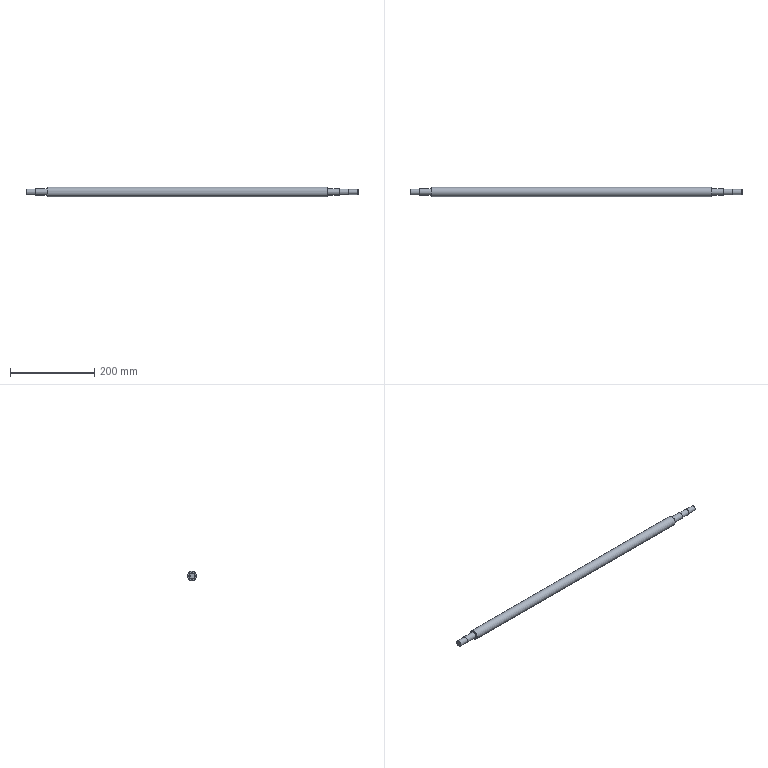Part | NX | 1 solid | 28 faces | box 787 x 22 x 22 mm | volume 271373 mm3 | plane 13 | cylinder 10 | cone 5 | commonest cylinder face diameters 5 x4 14 x2 15 x2 12 x1 22 x1
STEP:
#1=CARTESIAN_POINT('',(382.5,0.,-6.5));
#2=VERTEX_POINT('',#1);
#3=CARTESIAN_POINT('',(382.5,0.,0.));
#4=DIRECTION('',(1.,0.,0.));
#5=DIRECTION('',(0.,0.,-1.));
#6=AXIS2_PLACEMENT_3D('',#3,#4,#5);
#7=CIRCLE('',#6,6.5);
#8=EDGE_CURVE('',#2,#2,#7,.T.);
#9=ORIENTED_EDGE('',*,*,#8,.T.);
#10=EDGE_LOOP('',(#9));
#11=FACE_BOUND('',#10,.T.);
#12=CARTESIAN_POINT('',(382.5,0.,-6.));
#13=VERTEX_POINT('',#12);
#14=CARTESIAN_POINT('',(382.5,0.,0.));
#15=DIRECTION('',(1.,0.,0.));
#16=DIRECTION('',(0.,0.,-1.));
#17=AXIS2_PLACEMENT_3D('',#14,#15,#16);
#18=CIRCLE('',#17,6.);
#19=EDGE_CURVE('',#13,#13,#18,.T.);
#20=ORIENTED_EDGE('',*,*,#19,.F.);
#21=EDGE_LOOP('',(#20));
#22=FACE_BOUND('',#21,.T.);
#23=CARTESIAN_POINT('',(382.5,0.,0.));
#24=DIRECTION('',(1.,0.,0.));
#25=DIRECTION('',(0.,0.,-1.));
#26=AXIS2_PLACEMENT_3D('',#23,#24,#25);
#27=PLANE('',#26);
#28=ADVANCED_FACE('',(#11,#22),#27,.T.);
#29=CARTESIAN_POINT('',(382.,0.,-7.));
#30=VERTEX_POINT('',#29);
#31=CARTESIAN_POINT('',(382.,0.,0.));
#32=DIRECTION('',(1.,0.,0.));
#33=DIRECTION('',(0.,0.,-1.));
#34=AXIS2_PLACEMENT_3D('',#31,#32,#33);
#35=CIRCLE('',#34,7.);
#36=EDGE_CURVE('',#30,#30,#35,.F.);
#37=ORIENTED_EDGE('',*,*,#36,.T.);
#38=EDGE_LOOP('',(#37));
#39=FACE_BOUND('',#38,.T.);
#40=CARTESIAN_POINT('',(360.5,0.,-7.));
#41=VERTEX_POINT('',#40);
#42=CARTESIAN_POINT('',(360.5,0.,0.));
#43=DIRECTION('',(1.,0.,0.));
#44=DIRECTION('',(0.,0.,-1.));
#45=AXIS2_PLACEMENT_3D('',#42,#43,#44);
#46=CIRCLE('',#45,7.);
#47=EDGE_CURVE('',#41,#41,#46,.T.);
#48=ORIENTED_EDGE('',*,*,#47,.T.);
#49=EDGE_LOOP('',(#48));
#50=FACE_BOUND('',#49,.T.);
#51=CARTESIAN_POINT('',(363.5,6.538,-2.5));
#52=VERTEX_POINT('',#51);
#53=CARTESIAN_POINT('',(363.5,6.538,2.5));
#54=VERTEX_POINT('',#53);
#55=CARTESIAN_POINT('',(363.5,6.538,-2.5));
#56=CARTESIAN_POINT('',(362.834,6.538,-2.5));
#57=CARTESIAN_POINT('',(361.548,6.777,-1.958));
#58=CARTESIAN_POINT('',(360.726,7.111,-0.004587));
#59=CARTESIAN_POINT('',(361.547,6.777,1.96));
#60=CARTESIAN_POINT('',(362.833,6.538,2.5));
#61=CARTESIAN_POINT('',(363.5,6.538,2.5));
#62=B_SPLINE_CURVE_WITH_KNOTS('',3,(#55,#56,#57,#58,#59,#60,#61),.UNSPECIFIED.,.F.,.F.,(4,1,1,1,4),(0.,0.00197,0.003939,0.005909,0.007878),.UNSPECIFIED.);
#63=EDGE_CURVE('',#52,#54,#62,.T.);
#64=ORIENTED_EDGE('',*,*,#63,.F.);
#65=CARTESIAN_POINT('',(378.5,6.538,-2.5));
#66=VERTEX_POINT('',#65);
#67=CARTESIAN_POINT('',(382.5,6.538,-2.5));
#68=DIRECTION('',(-1.,0.,0.));
#69=VECTOR('',#68,1000.);
#70=LINE('',#67,#69);
#71=EDGE_CURVE('',#66,#52,#70,.T.);
#72=ORIENTED_EDGE('',*,*,#71,.F.);
#73=CARTESIAN_POINT('',(378.5,6.538,2.5));
#74=VERTEX_POINT('',#73);
#75=CARTESIAN_POINT('',(378.5,6.538,2.5));
#76=CARTESIAN_POINT('',(379.166,6.538,2.5));
#77=CARTESIAN_POINT('',(380.452,6.777,1.958));
#78=CARTESIAN_POINT('',(381.274,7.111,0.004587));
#79=CARTESIAN_POINT('',(380.453,6.777,-1.96));
#80=CARTESIAN_POINT('',(379.167,6.538,-2.5));
#81=CARTESIAN_POINT('',(378.5,6.538,-2.5));
#82=B_SPLINE_CURVE_WITH_KNOTS('',3,(#75,#76,#77,#78,#79,#80,#81),.UNSPECIFIED.,.F.,.F.,(4,1,1,1,4),(0.,0.00197,0.003939,0.005909,0.007878),.UNSPECIFIED.);
#83=EDGE_CURVE('',#74,#66,#82,.T.);
#84=ORIENTED_EDGE('',*,*,#83,.F.);
#85=CARTESIAN_POINT('',(382.5,6.538,2.5));
#86=DIRECTION('',(-1.,0.,0.));
#87=VECTOR('',#86,1000.);
#88=LINE('',#85,#87);
#89=EDGE_CURVE('',#54,#74,#88,.F.);
#90=ORIENTED_EDGE('',*,*,#89,.F.);
#91=EDGE_LOOP('',(#64,#72,#84,#90));
#92=FACE_BOUND('',#91,.T.);
#93=CARTESIAN_POINT('',(382.5,0.,0.));
#94=DIRECTION('',(-1.,0.,0.));
#95=DIRECTION('',(0.,0.,1.));
#96=AXIS2_PLACEMENT_3D('',#93,#94,#95);
#97=CYLINDRICAL_SURFACE('',#96,7.);
#98=ADVANCED_FACE('',(#39,#50,#92),#97,.T.);
#99=CARTESIAN_POINT('',(360.5,0.,-7.5));
#100=VERTEX_POINT('',#99);
#101=CARTESIAN_POINT('',(360.5,0.,0.));
#102=DIRECTION('',(1.,0.,0.));
#103=DIRECTION('',(0.,0.,-1.));
#104=AXIS2_PLACEMENT_3D('',#101,#102,#103);
#105=CIRCLE('',#104,7.5);
#106=EDGE_CURVE('',#100,#100,#105,.T.);
#107=ORIENTED_EDGE('',*,*,#106,.T.);
#108=EDGE_LOOP('',(#107));
#109=FACE_BOUND('',#108,.T.);
#110=ORIENTED_EDGE('',*,*,#47,.F.);
#111=EDGE_LOOP('',(#110));
#112=FACE_BOUND('',#111,.T.);
#113=CARTESIAN_POINT('',(360.5,0.,0.));
#114=DIRECTION('',(1.,0.,0.));
#115=DIRECTION('',(0.,0.,-1.));
#116=AXIS2_PLACEMENT_3D('',#113,#114,#115);
#117=PLANE('',#116);
#118=ADVANCED_FACE('',(#109,#112),#117,.T.);
#119=CARTESIAN_POINT('',(332.5,0.,-10.5));
#120=VERTEX_POINT('',#119);
#121=CARTESIAN_POINT('',(332.5,0.,0.));
#122=DIRECTION('',(1.,0.,0.));
#123=DIRECTION('',(0.,0.,-1.));
#124=AXIS2_PLACEMENT_3D('',#121,#122,#123);
#125=CIRCLE('',#124,10.5);
#126=EDGE_CURVE('',#120,#120,#125,.T.);
#127=ORIENTED_EDGE('',*,*,#126,.T.);
#128=EDGE_LOOP('',(#127));
#129=FACE_BOUND('',#128,.T.);
#130=CARTESIAN_POINT('',(332.5,0.,-7.5));
#131=VERTEX_POINT('',#130);
#132=CARTESIAN_POINT('',(332.5,0.,0.));
#133=DIRECTION('',(1.,0.,0.));
#134=DIRECTION('',(0.,0.,-1.));
#135=AXIS2_PLACEMENT_3D('',#132,#133,#134);
#136=CIRCLE('',#135,7.5);
#137=EDGE_CURVE('',#131,#131,#136,.T.);
#138=ORIENTED_EDGE('',*,*,#137,.F.);
#139=EDGE_LOOP('',(#138));
#140=FACE_BOUND('',#139,.T.);
#141=CARTESIAN_POINT('',(332.5,0.,0.));
#142=DIRECTION('',(1.,0.,0.));
#143=DIRECTION('',(0.,0.,-1.));
#144=AXIS2_PLACEMENT_3D('',#141,#142,#143);
#145=PLANE('',#144);
#146=ADVANCED_FACE('',(#129,#140),#145,.T.);
#147=CARTESIAN_POINT('',(-332.,0.,-11.));
#148=VERTEX_POINT('',#147);
#149=CARTESIAN_POINT('',(-332.,0.,0.));
#150=DIRECTION('',(1.,0.,0.));
#151=DIRECTION('',(0.,0.,-1.));
#152=AXIS2_PLACEMENT_3D('',#149,#150,#151);
#153=CIRCLE('',#152,11.);
#154=EDGE_CURVE('',#148,#148,#153,.T.);
#155=ORIENTED_EDGE('',*,*,#154,.T.);
#156=EDGE_LOOP('',(#155));
#157=FACE_BOUND('',#156,.T.);
#158=CARTESIAN_POINT('',(332.,0.,-11.));
#159=VERTEX_POINT('',#158);
#160=CARTESIAN_POINT('',(332.,0.,0.));
#161=DIRECTION('',(1.,0.,0.));
#162=DIRECTION('',(0.,0.,-1.));
#163=AXIS2_PLACEMENT_3D('',#160,#161,#162);
#164=CIRCLE('',#163,11.);
#165=EDGE_CURVE('',#159,#159,#164,.F.);
#166=ORIENTED_EDGE('',*,*,#165,.T.);
#167=EDGE_LOOP('',(#166));
#168=FACE_BOUND('',#167,.T.);
#169=CARTESIAN_POINT('',(332.5,0.,0.));
#170=DIRECTION('',(-1.,0.,0.));
#171=DIRECTION('',(0.,0.,1.));
#172=AXIS2_PLACEMENT_3D('',#169,#170,#171);
#173=CYLINDRICAL_SURFACE('',#172,11.);
#174=ADVANCED_FACE('',(#157,#168),#173,.T.);
#175=CARTESIAN_POINT('',(-332.5,0.,-10.5));
#176=VERTEX_POINT('',#175);
#177=CARTESIAN_POINT('',(-332.5,0.,0.));
#178=DIRECTION('',(1.,0.,0.));
#179=DIRECTION('',(0.,0.,-1.));
#180=AXIS2_PLACEMENT_3D('',#177,#178,#179);
#181=CIRCLE('',#180,10.5);
#182=EDGE_CURVE('',#176,#176,#181,.F.);
#183=ORIENTED_EDGE('',*,*,#182,.T.);
#184=EDGE_LOOP('',(#183));
#185=FACE_BOUND('',#184,.T.);
#186=CARTESIAN_POINT('',(-332.5,0.,-7.5));
#187=VERTEX_POINT('',#186);
#188=CARTESIAN_POINT('',(-332.5,0.,0.));
#189=DIRECTION('',(1.,0.,0.));
#190=DIRECTION('',(0.,0.,-1.));
#191=AXIS2_PLACEMENT_3D('',#188,#189,#190);
#192=CIRCLE('',#191,7.5);
#193=EDGE_CURVE('',#187,#187,#192,.T.);
#194=ORIENTED_EDGE('',*,*,#193,.T.);
#195=EDGE_LOOP('',(#194));
#196=FACE_BOUND('',#195,.T.);
#197=CARTESIAN_POINT('',(-332.5,0.,0.));
#198=DIRECTION('',(1.,0.,0.));
#199=DIRECTION('',(0.,0.,-1.));
#200=AXIS2_PLACEMENT_3D('',#197,#198,#199);
#201=PLANE('',#200);
#202=ADVANCED_FACE('',(#185,#196),#201,.F.);
#203=ORIENTED_EDGE('',*,*,#106,.F.);
#204=EDGE_LOOP('',(#203));
#205=FACE_BOUND('',#204,.T.);
#206=ORIENTED_EDGE('',*,*,#137,.T.);
#207=EDGE_LOOP('',(#206));
#208=FACE_BOUND('',#207,.T.);
#209=CARTESIAN_POINT('',(360.5,0.,0.));
#210=DIRECTION('',(-1.,0.,0.));
#211=DIRECTION('',(0.,0.,1.));
#212=AXIS2_PLACEMENT_3D('',#209,#210,#211);
#213=CYLINDRICAL_SURFACE('',#212,7.5);
#214=ADVANCED_FACE('',(#205,#208),#213,.T.);
#215=CARTESIAN_POINT('',(378.5,4.,2.5));
#216=VERTEX_POINT('',#215);
#217=CARTESIAN_POINT('',(378.5,4.,2.5));
#218=DIRECTION('',(0.,1.,0.));
#219=VECTOR('',#218,1000.);
#220=LINE('',#217,#219);
#221=EDGE_CURVE('',#216,#74,#220,.T.);
#222=ORIENTED_EDGE('',*,*,#221,.T.);
#223=ORIENTED_EDGE('',*,*,#83,.T.);
#224=CARTESIAN_POINT('',(378.5,4.,-2.5));
#225=VERTEX_POINT('',#224);
#226=CARTESIAN_POINT('',(378.5,4.,-2.5));
#227=DIRECTION('',(0.,1.,0.));
#228=VECTOR('',#227,1000.);
#229=LINE('',#226,#228);
#230=EDGE_CURVE('',#225,#66,#229,.T.);
#231=ORIENTED_EDGE('',*,*,#230,.F.);
#232=CARTESIAN_POINT('',(378.5,4.,0.));
#233=DIRECTION('',(0.,-1.,0.));
#234=DIRECTION('',(0.,0.,1.));
#235=AXIS2_PLACEMENT_3D('',#232,#233,#234);
#236=CIRCLE('',#235,2.5);
#237=EDGE_CURVE('',#225,#216,#236,.T.);
#238=ORIENTED_EDGE('',*,*,#237,.T.);
#239=EDGE_LOOP('',(#222,#223,#231,#238));
#240=FACE_BOUND('',#239,.T.);
#241=CARTESIAN_POINT('',(378.5,4.,0.));
#242=DIRECTION('',(0.,1.,0.));
#243=DIRECTION('',(0.,0.,1.));
#244=AXIS2_PLACEMENT_3D('',#241,#242,#243);
#245=CYLINDRICAL_SURFACE('',#244,2.5);
#246=ADVANCED_FACE('',(#240),#245,.F.);
#247=ORIENTED_EDGE('',*,*,#89,.T.);
#248=ORIENTED_EDGE('',*,*,#221,.F.);
#249=CARTESIAN_POINT('',(363.5,4.,2.5));
#250=VERTEX_POINT('',#249);
#251=CARTESIAN_POINT('',(378.5,4.,2.5));
#252=DIRECTION('',(-1.,0.,0.));
#253=VECTOR('',#252,1000.);
#254=LINE('',#251,#253);
#255=EDGE_CURVE('',#216,#250,#254,.T.);
#256=ORIENTED_EDGE('',*,*,#255,.T.);
#257=CARTESIAN_POINT('',(363.5,4.,2.5));
#258=DIRECTION('',(0.,1.,0.));
#259=VECTOR('',#258,1000.);
#260=LINE('',#257,#259);
#261=EDGE_CURVE('',#250,#54,#260,.T.);
#262=ORIENTED_EDGE('',*,*,#261,.T.);
#263=EDGE_LOOP('',(#247,#248,#256,#262));
#264=FACE_BOUND('',#263,.T.);
#265=CARTESIAN_POINT('',(378.5,4.,2.5));
#266=DIRECTION('',(0.,0.,-1.));
#267=DIRECTION('',(0.,1.,0.));
#268=AXIS2_PLACEMENT_3D('',#265,#266,#267);
#269=PLANE('',#268);
#270=ADVANCED_FACE('',(#264),#269,.T.);
#271=CARTESIAN_POINT('',(363.5,4.,-2.5));
#272=VERTEX_POINT('',#271);
#273=CARTESIAN_POINT('',(363.5,4.,-2.5));
#274=DIRECTION('',(0.,1.,0.));
#275=VECTOR('',#274,1000.);
#276=LINE('',#273,#275);
#277=EDGE_CURVE('',#272,#52,#276,.T.);
#278=ORIENTED_EDGE('',*,*,#277,.T.);
#279=ORIENTED_EDGE('',*,*,#63,.T.);
#280=ORIENTED_EDGE('',*,*,#261,.F.);
#281=CARTESIAN_POINT('',(363.5,4.,0.));
#282=DIRECTION('',(0.,-1.,0.));
#283=DIRECTION('',(0.,0.,-1.));
#284=AXIS2_PLACEMENT_3D('',#281,#282,#283);
#285=CIRCLE('',#284,2.5);
#286=EDGE_CURVE('',#250,#272,#285,.T.);
#287=ORIENTED_EDGE('',*,*,#286,.T.);
#288=EDGE_LOOP('',(#278,#279,#280,#287));
#289=FACE_BOUND('',#288,.T.);
#290=CARTESIAN_POINT('',(363.5,4.,0.));
#291=DIRECTION('',(0.,1.,0.));
#292=DIRECTION('',(0.,0.,1.));
#293=AXIS2_PLACEMENT_3D('',#290,#291,#292);
#294=CYLINDRICAL_SURFACE('',#293,2.5);
#295=ADVANCED_FACE('',(#289),#294,.F.);
#296=ORIENTED_EDGE('',*,*,#71,.T.);
#297=ORIENTED_EDGE('',*,*,#277,.F.);
#298=CARTESIAN_POINT('',(378.5,4.,-2.5));
#299=DIRECTION('',(1.,0.,0.));
#300=VECTOR('',#299,1000.);
#301=LINE('',#298,#300);
#302=EDGE_CURVE('',#272,#225,#301,.T.);
#303=ORIENTED_EDGE('',*,*,#302,.T.);
#304=ORIENTED_EDGE('',*,*,#230,.T.);
#305=EDGE_LOOP('',(#296,#297,#303,#304));
#306=FACE_BOUND('',#305,.T.);
#307=CARTESIAN_POINT('',(378.5,4.,-2.5));
#308=DIRECTION('',(0.,0.,1.));
#309=DIRECTION('',(0.,-1.,0.));
#310=AXIS2_PLACEMENT_3D('',#307,#308,#309);
#311=PLANE('',#310);
#312=ADVANCED_FACE('',(#306),#311,.T.);
#313=ORIENTED_EDGE('',*,*,#237,.F.);
#314=ORIENTED_EDGE('',*,*,#302,.F.);
#315=ORIENTED_EDGE('',*,*,#286,.F.);
#316=ORIENTED_EDGE('',*,*,#255,.F.);
#317=EDGE_LOOP('',(#313,#314,#315,#316));
#318=FACE_BOUND('',#317,.T.);
#319=CARTESIAN_POINT('',(378.5,4.,0.));
#320=DIRECTION('',(0.,1.,0.));
#321=DIRECTION('',(0.,0.,1.));
#322=AXIS2_PLACEMENT_3D('',#319,#320,#321);
#323=PLANE('',#322);
#324=ADVANCED_FACE('',(#318),#323,.T.);
#325=CARTESIAN_POINT('',(-360.5,0.,-7.5));
#326=VERTEX_POINT('',#325);
#327=CARTESIAN_POINT('',(-360.5,0.,0.));
#328=DIRECTION('',(1.,0.,0.));
#329=DIRECTION('',(0.,0.,-1.));
#330=AXIS2_PLACEMENT_3D('',#327,#328,#329);
#331=CIRCLE('',#330,7.5);
#332=EDGE_CURVE('',#326,#326,#331,.T.);
#333=ORIENTED_EDGE('',*,*,#332,.T.);
#334=EDGE_LOOP('',(#333));
#335=FACE_BOUND('',#334,.T.);
#336=ORIENTED_EDGE('',*,*,#193,.F.);
#337=EDGE_LOOP('',(#336));
#338=FACE_BOUND('',#337,.T.);
#339=CARTESIAN_POINT('',(-360.5,0.,0.));
#340=DIRECTION('',(1.,0.,0.));
#341=DIRECTION('',(0.,0.,-1.));
#342=AXIS2_PLACEMENT_3D('',#339,#340,#341);
#343=CYLINDRICAL_SURFACE('',#342,7.5);
#344=ADVANCED_FACE('',(#335,#338),#343,.T.);
#345=CARTESIAN_POINT('',(-360.5,0.,7.));
#346=VERTEX_POINT('',#345);
#347=CARTESIAN_POINT('',(-360.5,0.,0.));
#348=DIRECTION('',(-1.,0.,0.));
#349=DIRECTION('',(0.,0.,1.));
#350=AXIS2_PLACEMENT_3D('',#347,#348,#349);
#351=CIRCLE('',#350,7.);
#352=EDGE_CURVE('',#346,#346,#351,.T.);
#353=ORIENTED_EDGE('',*,*,#352,.F.);
#354=EDGE_LOOP('',(#353));
#355=FACE_BOUND('',#354,.T.);
#356=ORIENTED_EDGE('',*,*,#332,.F.);
#357=EDGE_LOOP('',(#356));
#358=FACE_BOUND('',#357,.T.);
#359=CARTESIAN_POINT('',(-360.5,0.,0.));
#360=DIRECTION('',(-1.,0.,0.));
#361=DIRECTION('',(0.,0.,-1.));
#362=AXIS2_PLACEMENT_3D('',#359,#360,#361);
#363=PLANE('',#362);
#364=ADVANCED_FACE('',(#355,#358),#363,.T.);
#365=CARTESIAN_POINT('',(-382.,0.,7.));
#366=VERTEX_POINT('',#365);
#367=CARTESIAN_POINT('',(-382.,0.,0.));
#368=DIRECTION('',(-1.,0.,0.));
#369=DIRECTION('',(0.,0.,1.));
#370=AXIS2_PLACEMENT_3D('',#367,#368,#369);
#371=CIRCLE('',#370,7.);
#372=EDGE_CURVE('',#366,#366,#371,.F.);
#373=ORIENTED_EDGE('',*,*,#372,.T.);
#374=EDGE_LOOP('',(#373));
#375=FACE_BOUND('',#374,.T.);
#376=CARTESIAN_POINT('',(-363.5,6.538,2.5));
#377=VERTEX_POINT('',#376);
#378=CARTESIAN_POINT('',(-363.5,6.538,-2.5));
#379=VERTEX_POINT('',#378);
#380=CARTESIAN_POINT('',(-363.5,6.538,2.5));
#381=CARTESIAN_POINT('',(-362.834,6.538,2.5));
#382=CARTESIAN_POINT('',(-361.548,6.777,1.958));
#383=CARTESIAN_POINT('',(-360.726,7.111,0.004587));
#384=CARTESIAN_POINT('',(-361.547,6.777,-1.96));
#385=CARTESIAN_POINT('',(-362.833,6.538,-2.5));
#386=CARTESIAN_POINT('',(-363.5,6.538,-2.5));
#387=B_SPLINE_CURVE_WITH_KNOTS('',3,(#380,#381,#382,#383,#384,#385,#386),.UNSPECIFIED.,.F.,.F.,(4,1,1,1,4),(0.,0.00197,0.003939,0.005909,0.007878),.UNSPECIFIED.);
#388=EDGE_CURVE('',#377,#379,#387,.T.);
#389=ORIENTED_EDGE('',*,*,#388,.F.);
#390=CARTESIAN_POINT('',(-378.5,6.538,2.5));
#391=VERTEX_POINT('',#390);
#392=CARTESIAN_POINT('',(-382.5,6.538,2.5));
#393=DIRECTION('',(1.,0.,0.));
#394=VECTOR('',#393,1000.);
#395=LINE('',#392,#394);
#396=EDGE_CURVE('',#391,#377,#395,.T.);
#397=ORIENTED_EDGE('',*,*,#396,.F.);
#398=CARTESIAN_POINT('',(-378.5,6.538,-2.5));
#399=VERTEX_POINT('',#398);
#400=CARTESIAN_POINT('',(-378.5,6.538,-2.5));
#401=CARTESIAN_POINT('',(-379.166,6.538,-2.5));
#402=CARTESIAN_POINT('',(-380.452,6.777,-1.958));
#403=CARTESIAN_POINT('',(-381.274,7.111,-0.004587));
#404=CARTESIAN_POINT('',(-380.453,6.777,1.96));
#405=CARTESIAN_POINT('',(-379.167,6.538,2.5));
#406=CARTESIAN_POINT('',(-378.5,6.538,2.5));
#407=B_SPLINE_CURVE_WITH_KNOTS('',3,(#400,#401,#402,#403,#404,#405,#406),.UNSPECIFIED.,.F.,.F.,(4,1,1,1,4),(0.,0.00197,0.003939,0.005909,0.007878),.UNSPECIFIED.);
#408=EDGE_CURVE('',#399,#391,#407,.T.);
#409=ORIENTED_EDGE('',*,*,#408,.F.);
#410=CARTESIAN_POINT('',(-382.5,6.538,-2.5));
#411=DIRECTION('',(1.,0.,0.));
#412=VECTOR('',#411,1000.);
#413=LINE('',#410,#412);
#414=EDGE_CURVE('',#379,#399,#413,.F.);
#415=ORIENTED_EDGE('',*,*,#414,.F.);
#416=EDGE_LOOP('',(#389,#397,#409,#415));
#417=FACE_BOUND('',#416,.T.);
#418=ORIENTED_EDGE('',*,*,#352,.T.);
#419=EDGE_LOOP('',(#418));
#420=FACE_BOUND('',#419,.T.);
#421=CARTESIAN_POINT('',(-382.5,0.,0.));
#422=DIRECTION('',(1.,0.,0.));
#423=DIRECTION('',(0.,0.,-1.));
#424=AXIS2_PLACEMENT_3D('',#421,#422,#423);
#425=CYLINDRICAL_SURFACE('',#424,7.);
#426=ADVANCED_FACE('',(#375,#417,#420),#425,.T.);
#427=CARTESIAN_POINT('',(-382.5,0.,6.5));
#428=VERTEX_POINT('',#427);
#429=CARTESIAN_POINT('',(-382.5,0.,0.));
#430=DIRECTION('',(-1.,0.,0.));
#431=DIRECTION('',(0.,0.,1.));
#432=AXIS2_PLACEMENT_3D('',#429,#430,#431);
#433=CIRCLE('',#432,6.5);
#434=EDGE_CURVE('',#428,#428,#433,.T.);
#435=ORIENTED_EDGE('',*,*,#434,.T.);
#436=EDGE_LOOP('',(#435));
#437=FACE_BOUND('',#436,.T.);
#438=CARTESIAN_POINT('',(-382.5,0.,0.));
#439=DIRECTION('',(-1.,0.,0.));
#440=DIRECTION('',(0.,0.,-1.));
#441=AXIS2_PLACEMENT_3D('',#438,#439,#440);
#442=PLANE('',#441);
#443=ADVANCED_FACE('',(#437),#442,.T.);
#444=CARTESIAN_POINT('',(-378.5,4.,-2.5));
#445=VERTEX_POINT('',#444);
#446=CARTESIAN_POINT('',(-378.5,4.,-2.5));
#447=DIRECTION('',(0.,1.,0.));
#448=VECTOR('',#447,1000.);
#449=LINE('',#446,#448);
#450=EDGE_CURVE('',#445,#399,#449,.T.);
#451=ORIENTED_EDGE('',*,*,#450,.T.);
#452=ORIENTED_EDGE('',*,*,#408,.T.);
#453=CARTESIAN_POINT('',(-378.5,4.,2.5));
#454=VERTEX_POINT('',#453);
#455=CARTESIAN_POINT('',(-378.5,4.,2.5));
#456=DIRECTION('',(0.,1.,0.));
#457=VECTOR('',#456,1000.);
#458=LINE('',#455,#457);
#459=EDGE_CURVE('',#454,#391,#458,.T.);
#460=ORIENTED_EDGE('',*,*,#459,.F.);
#461=CARTESIAN_POINT('',(-378.5,4.,0.));
#462=DIRECTION('',(0.,1.,0.));
#463=DIRECTION('',(0.,0.,1.));
#464=AXIS2_PLACEMENT_3D('',#461,#462,#463);
#465=CIRCLE('',#464,2.5);
#466=EDGE_CURVE('',#445,#454,#465,.T.);
#467=ORIENTED_EDGE('',*,*,#466,.F.);
#468=EDGE_LOOP('',(#451,#452,#460,#467));
#469=FACE_BOUND('',#468,.T.);
#470=CARTESIAN_POINT('',(-378.5,4.,0.));
#471=DIRECTION('',(0.,1.,0.));
#472=DIRECTION('',(0.,0.,1.));
#473=AXIS2_PLACEMENT_3D('',#470,#471,#472);
#474=CYLINDRICAL_SURFACE('',#473,2.5);
#475=ADVANCED_FACE('',(#469),#474,.F.);
#476=ORIENTED_EDGE('',*,*,#414,.T.);
#477=ORIENTED_EDGE('',*,*,#450,.F.);
#478=CARTESIAN_POINT('',(-363.5,4.,-2.5));
#479=VERTEX_POINT('',#478);
#480=CARTESIAN_POINT('',(-378.5,4.,-2.5));
#481=DIRECTION('',(-1.,0.,0.));
#482=VECTOR('',#481,1000.);
#483=LINE('',#480,#482);
#484=EDGE_CURVE('',#479,#445,#483,.T.);
#485=ORIENTED_EDGE('',*,*,#484,.F.);
#486=CARTESIAN_POINT('',(-363.5,4.,-2.5));
#487=DIRECTION('',(0.,1.,0.));
#488=VECTOR('',#487,1000.);
#489=LINE('',#486,#488);
#490=EDGE_CURVE('',#479,#379,#489,.T.);
#491=ORIENTED_EDGE('',*,*,#490,.T.);
#492=EDGE_LOOP('',(#476,#477,#485,#491));
#493=FACE_BOUND('',#492,.T.);
#494=CARTESIAN_POINT('',(-378.5,4.,-2.5));
#495=DIRECTION('',(0.,0.,-1.));
#496=DIRECTION('',(0.,1.,0.));
#497=AXIS2_PLACEMENT_3D('',#494,#495,#496);
#498=PLANE('',#497);
#499=ADVANCED_FACE('',(#493),#498,.F.);
#500=CARTESIAN_POINT('',(-363.5,4.,2.5));
#501=VERTEX_POINT('',#500);
#502=CARTESIAN_POINT('',(-363.5,4.,2.5));
#503=DIRECTION('',(0.,1.,0.));
#504=VECTOR('',#503,1000.);
#505=LINE('',#502,#504);
#506=EDGE_CURVE('',#501,#377,#505,.T.);
#507=ORIENTED_EDGE('',*,*,#506,.T.);
#508=ORIENTED_EDGE('',*,*,#388,.T.);
#509=ORIENTED_EDGE('',*,*,#490,.F.);
#510=CARTESIAN_POINT('',(-363.5,4.,0.));
#511=DIRECTION('',(0.,1.,0.));
#512=DIRECTION('',(0.,0.,-1.));
#513=AXIS2_PLACEMENT_3D('',#510,#511,#512);
#514=CIRCLE('',#513,2.5);
#515=EDGE_CURVE('',#501,#479,#514,.T.);
#516=ORIENTED_EDGE('',*,*,#515,.F.);
#517=EDGE_LOOP('',(#507,#508,#509,#516));
#518=FACE_BOUND('',#517,.T.);
#519=CARTESIAN_POINT('',(-363.5,4.,0.));
#520=DIRECTION('',(0.,1.,0.));
#521=DIRECTION('',(0.,0.,1.));
#522=AXIS2_PLACEMENT_3D('',#519,#520,#521);
#523=CYLINDRICAL_SURFACE('',#522,2.5);
#524=ADVANCED_FACE('',(#518),#523,.F.);
#525=ORIENTED_EDGE('',*,*,#396,.T.);
#526=ORIENTED_EDGE('',*,*,#506,.F.);
#527=CARTESIAN_POINT('',(-378.5,4.,2.5));
#528=DIRECTION('',(1.,0.,0.));
#529=VECTOR('',#528,1000.);
#530=LINE('',#527,#529);
#531=EDGE_CURVE('',#454,#501,#530,.T.);
#532=ORIENTED_EDGE('',*,*,#531,.F.);
#533=ORIENTED_EDGE('',*,*,#459,.T.);
#534=EDGE_LOOP('',(#525,#526,#532,#533));
#535=FACE_BOUND('',#534,.T.);
#536=CARTESIAN_POINT('',(-378.5,4.,2.5));
#537=DIRECTION('',(0.,0.,1.));
#538=DIRECTION('',(0.,-1.,0.));
#539=AXIS2_PLACEMENT_3D('',#536,#537,#538);
#540=PLANE('',#539);
#541=ADVANCED_FACE('',(#535),#540,.F.);
#542=ORIENTED_EDGE('',*,*,#466,.T.);
#543=ORIENTED_EDGE('',*,*,#531,.T.);
#544=ORIENTED_EDGE('',*,*,#515,.T.);
#545=ORIENTED_EDGE('',*,*,#484,.T.);
#546=EDGE_LOOP('',(#542,#543,#544,#545));
#547=FACE_BOUND('',#546,.T.);
#548=CARTESIAN_POINT('',(-378.5,4.,0.));
#549=DIRECTION('',(0.,1.,0.));
#550=DIRECTION('',(0.,0.,1.));
#551=AXIS2_PLACEMENT_3D('',#548,#549,#550);
#552=PLANE('',#551);
#553=ADVANCED_FACE('',(#547),#552,.T.);
#554=CARTESIAN_POINT('',(404.,0.,-6.));
#555=VERTEX_POINT('',#554);
#556=CARTESIAN_POINT('',(404.,0.,0.));
#557=DIRECTION('',(1.,0.,0.));
#558=DIRECTION('',(0.,0.,-1.));
#559=AXIS2_PLACEMENT_3D('',#556,#557,#558);
#560=CIRCLE('',#559,6.);
#561=EDGE_CURVE('',#555,#555,#560,.F.);
#562=ORIENTED_EDGE('',*,*,#561,.T.);
#563=EDGE_LOOP('',(#562));
#564=FACE_BOUND('',#563,.T.);
#565=ORIENTED_EDGE('',*,*,#19,.T.);
#566=EDGE_LOOP('',(#565));
#567=FACE_BOUND('',#566,.T.);
#568=CARTESIAN_POINT('',(404.5,0.,0.));
#569=DIRECTION('',(-1.,0.,0.));
#570=DIRECTION('',(0.,0.,1.));
#571=AXIS2_PLACEMENT_3D('',#568,#569,#570);
#572=CYLINDRICAL_SURFACE('',#571,6.);
#573=ADVANCED_FACE('',(#564,#567),#572,.T.);
#574=CARTESIAN_POINT('',(404.5,0.,-5.5));
#575=VERTEX_POINT('',#574);
#576=CARTESIAN_POINT('',(404.5,0.,0.));
#577=DIRECTION('',(1.,0.,0.));
#578=DIRECTION('',(0.,0.,-1.));
#579=AXIS2_PLACEMENT_3D('',#576,#577,#578);
#580=CIRCLE('',#579,5.5);
#581=EDGE_CURVE('',#575,#575,#580,.T.);
#582=ORIENTED_EDGE('',*,*,#581,.T.);
#583=EDGE_LOOP('',(#582));
#584=FACE_BOUND('',#583,.T.);
#585=CARTESIAN_POINT('',(404.5,0.,0.));
#586=DIRECTION('',(1.,0.,0.));
#587=DIRECTION('',(0.,0.,-1.));
#588=AXIS2_PLACEMENT_3D('',#585,#586,#587);
#589=PLANE('',#588);
#590=ADVANCED_FACE('',(#584),#589,.T.);
#591=ORIENTED_EDGE('',*,*,#561,.F.);
#592=EDGE_LOOP('',(#591));
#593=FACE_BOUND('',#592,.T.);
#594=ORIENTED_EDGE('',*,*,#581,.F.);
#595=EDGE_LOOP('',(#594));
#596=FACE_BOUND('',#595,.T.);
#597=CARTESIAN_POINT('',(404.5,0.,0.));
#598=DIRECTION('',(-1.,0.,0.));
#599=DIRECTION('',(0.,0.,1.));
#600=AXIS2_PLACEMENT_3D('',#597,#598,#599);
#601=CONICAL_SURFACE('',#600,5.5,0.7854);
#602=ADVANCED_FACE('',(#593,#596),#601,.T.);
#603=ORIENTED_EDGE('',*,*,#434,.F.);
#604=EDGE_LOOP('',(#603));
#605=FACE_BOUND('',#604,.T.);
#606=ORIENTED_EDGE('',*,*,#372,.F.);
#607=EDGE_LOOP('',(#606));
#608=FACE_BOUND('',#607,.T.);
#609=CARTESIAN_POINT('',(-382.,0.,0.));
#610=DIRECTION('',(1.,0.,0.));
#611=DIRECTION('',(0.,0.,-1.));
#612=AXIS2_PLACEMENT_3D('',#609,#610,#611);
#613=CONICAL_SURFACE('',#612,7.,0.7854);
#614=ADVANCED_FACE('',(#605,#608),#613,.T.);
#615=ORIENTED_EDGE('',*,*,#182,.F.);
#616=EDGE_LOOP('',(#615));
#617=FACE_BOUND('',#616,.T.);
#618=ORIENTED_EDGE('',*,*,#154,.F.);
#619=EDGE_LOOP('',(#618));
#620=FACE_BOUND('',#619,.T.);
#621=CARTESIAN_POINT('',(-332.,0.,0.));
#622=DIRECTION('',(1.,0.,0.));
#623=DIRECTION('',(0.,0.,-1.));
#624=AXIS2_PLACEMENT_3D('',#621,#622,#623);
#625=CONICAL_SURFACE('',#624,11.,0.7854);
#626=ADVANCED_FACE('',(#617,#620),#625,.T.);
#627=ORIENTED_EDGE('',*,*,#165,.F.);
#628=EDGE_LOOP('',(#627));
#629=FACE_BOUND('',#628,.T.);
#630=ORIENTED_EDGE('',*,*,#126,.F.);
#631=EDGE_LOOP('',(#630));
#632=FACE_BOUND('',#631,.T.);
#633=CARTESIAN_POINT('',(332.5,0.,0.));
#634=DIRECTION('',(-1.,0.,0.));
#635=DIRECTION('',(0.,0.,1.));
#636=AXIS2_PLACEMENT_3D('',#633,#634,#635);
#637=CONICAL_SURFACE('',#636,10.5,0.7854);
#638=ADVANCED_FACE('',(#629,#632),#637,.T.);
#639=ORIENTED_EDGE('',*,*,#36,.F.);
#640=EDGE_LOOP('',(#639));
#641=FACE_BOUND('',#640,.T.);
#642=ORIENTED_EDGE('',*,*,#8,.F.);
#643=EDGE_LOOP('',(#642));
#644=FACE_BOUND('',#643,.T.);
#645=CARTESIAN_POINT('',(382.5,0.,0.));
#646=DIRECTION('',(-1.,0.,0.));
#647=DIRECTION('',(0.,0.,1.));
#648=AXIS2_PLACEMENT_3D('',#645,#646,#647);
#649=CONICAL_SURFACE('',#648,6.5,0.7854);
#650=ADVANCED_FACE('',(#641,#644),#649,.T.);
#651=CLOSED_SHELL('',(#28,#98,#118,#146,#174,#202,#214,#246,#270,#295,#312,#324,#344,#364,#426,#443,#475,#499,#524,#541,#553,#573,#590,#602,#614,#626,#638,#650));
#652=MANIFOLD_SOLID_BREP('',#651);
#653=(LENGTH_UNIT()NAMED_UNIT(*)SI_UNIT(.MILLI.,.METRE.));
#654=UNCERTAINTY_MEASURE_WITH_UNIT(LENGTH_MEASURE(0.0508),#653,'','');
#655=(NAMED_UNIT(*)PLANE_ANGLE_UNIT()SI_UNIT($,.RADIAN.));
#656=(NAMED_UNIT(*)SI_UNIT($,.STERADIAN.)SOLID_ANGLE_UNIT());
#657=(GEOMETRIC_REPRESENTATION_CONTEXT(3)GLOBAL_UNCERTAINTY_ASSIGNED_CONTEXT((#654))GLOBAL_UNIT_ASSIGNED_CONTEXT((#653,#655,#656))REPRESENTATION_CONTEXT('',''));
#658=ADVANCED_BREP_SHAPE_REPRESENTATION('',(#652),#657);